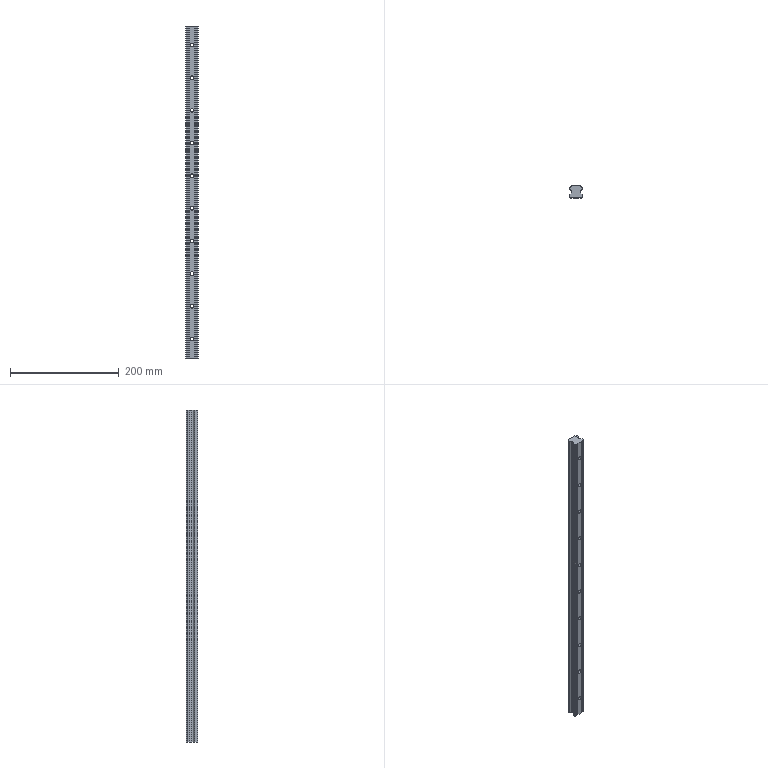Part | SolidWorks | features ICE 3, BaseBody 1, HoleWzd 1, LPattern 1 | 1 solid | 84 faces | box 23 x 22 x 610 mm | volume 256299 mm3 | cylinder 44 | plane 40 | commonest cylinder face diameters 11 x20 6.6 x14 7 x6 4.6 x4